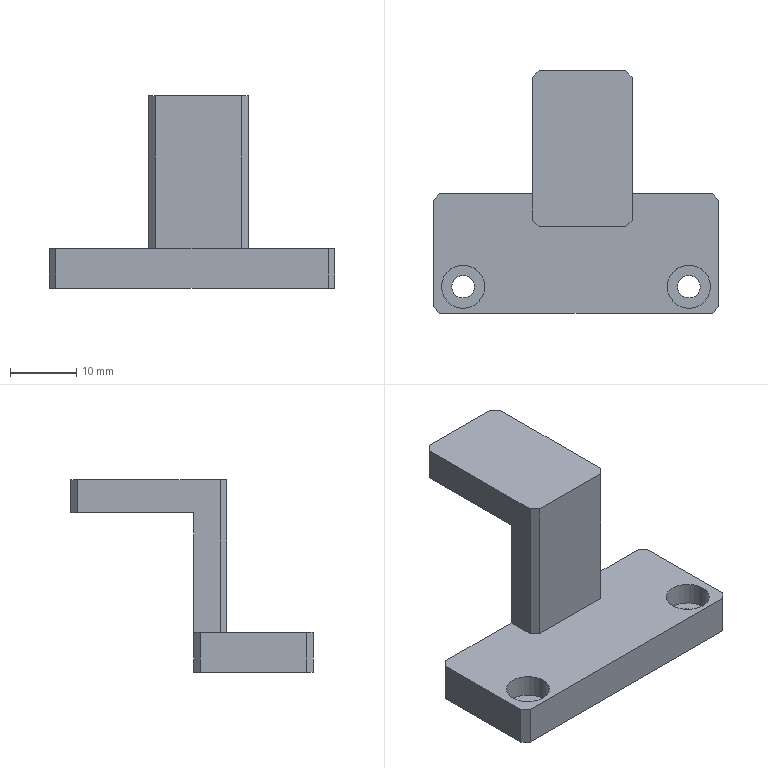Part | NX | 1 solid | 26 faces | box 43 x 36.5 x 29 mm | volume 7444 mm3 | plane 22 | cylinder 4 | commonest cylinder face diameters 3.4 x2 6.5 x2
STEP:
#1=CARTESIAN_POINT('',(21.5,8.,5.));
#2=VERTEX_POINT('',#1);
#3=CARTESIAN_POINT('',(20.5,9.,5.));
#4=VERTEX_POINT('',#3);
#5=CARTESIAN_POINT('',(14.75,14.75,5.));
#6=DIRECTION('',(-0.7071,0.7071,0.));
#7=VECTOR('',#6,1000.);
#8=LINE('',#5,#7);
#9=EDGE_CURVE('',#2,#4,#8,.T.);
#10=ORIENTED_EDGE('',*,*,#9,.F.);
#11=CARTESIAN_POINT('',(21.5,8.,-1.));
#12=VERTEX_POINT('',#11);
#13=CARTESIAN_POINT('',(21.5,8.,5.));
#14=DIRECTION('',(0.,0.,1.));
#15=VECTOR('',#14,1000.);
#16=LINE('',#13,#15);
#17=EDGE_CURVE('',#12,#2,#16,.T.);
#18=ORIENTED_EDGE('',*,*,#17,.F.);
#19=CARTESIAN_POINT('',(20.5,9.,-1.));
#20=VERTEX_POINT('',#19);
#21=CARTESIAN_POINT('',(20.5,9.,-1.));
#22=DIRECTION('',(0.7071,-0.7071,0.));
#23=VECTOR('',#22,1000.);
#24=LINE('',#21,#23);
#25=EDGE_CURVE('',#20,#12,#24,.T.);
#26=ORIENTED_EDGE('',*,*,#25,.F.);
#27=CARTESIAN_POINT('',(20.5,9.,5.));
#28=DIRECTION('',(0.,0.,-1.));
#29=VECTOR('',#28,1000.);
#30=LINE('',#27,#29);
#31=EDGE_CURVE('',#4,#20,#30,.T.);
#32=ORIENTED_EDGE('',*,*,#31,.F.);
#33=EDGE_LOOP('',(#10,#18,#26,#32));
#34=FACE_BOUND('',#33,.T.);
#35=CARTESIAN_POINT('',(20.5,9.,5.));
#36=DIRECTION('',(-0.7071,-0.7071,0.));
#37=DIRECTION('',(0.,0.,-1.));
#38=AXIS2_PLACEMENT_3D('',#35,#36,#37);
#39=PLANE('',#38);
#40=ADVANCED_FACE('',(#34),#39,.F.);
#41=CARTESIAN_POINT('',(20.5,-9.,5.));
#42=VERTEX_POINT('',#41);
#43=CARTESIAN_POINT('',(21.5,-8.,5.));
#44=VERTEX_POINT('',#43);
#45=CARTESIAN_POINT('',(14.75,-14.75,5.));
#46=DIRECTION('',(0.7071,0.7071,0.));
#47=VECTOR('',#46,1000.);
#48=LINE('',#45,#47);
#49=EDGE_CURVE('',#42,#44,#48,.T.);
#50=ORIENTED_EDGE('',*,*,#49,.F.);
#51=CARTESIAN_POINT('',(20.5,-9.,-1.));
#52=VERTEX_POINT('',#51);
#53=CARTESIAN_POINT('',(20.5,-9.,5.));
#54=DIRECTION('',(0.,0.,1.));
#55=VECTOR('',#54,1000.);
#56=LINE('',#53,#55);
#57=EDGE_CURVE('',#52,#42,#56,.T.);
#58=ORIENTED_EDGE('',*,*,#57,.F.);
#59=CARTESIAN_POINT('',(21.5,-8.,-1.));
#60=VERTEX_POINT('',#59);
#61=CARTESIAN_POINT('',(21.5,-8.,-1.));
#62=DIRECTION('',(-0.7071,-0.7071,0.));
#63=VECTOR('',#62,1000.);
#64=LINE('',#61,#63);
#65=EDGE_CURVE('',#60,#52,#64,.T.);
#66=ORIENTED_EDGE('',*,*,#65,.F.);
#67=CARTESIAN_POINT('',(21.5,-8.,5.));
#68=DIRECTION('',(0.,0.,-1.));
#69=VECTOR('',#68,1000.);
#70=LINE('',#67,#69);
#71=EDGE_CURVE('',#44,#60,#70,.T.);
#72=ORIENTED_EDGE('',*,*,#71,.F.);
#73=EDGE_LOOP('',(#50,#58,#66,#72));
#74=FACE_BOUND('',#73,.T.);
#75=CARTESIAN_POINT('',(21.5,-8.,5.));
#76=DIRECTION('',(-0.7071,0.7071,0.));
#77=DIRECTION('',(0.,0.,-1.));
#78=AXIS2_PLACEMENT_3D('',#75,#76,#77);
#79=PLANE('',#78);
#80=ADVANCED_FACE('',(#74),#79,.F.);
#81=CARTESIAN_POINT('',(-20.5,9.,5.));
#82=VERTEX_POINT('',#81);
#83=CARTESIAN_POINT('',(-21.5,8.,5.));
#84=VERTEX_POINT('',#83);
#85=CARTESIAN_POINT('',(-14.75,14.75,5.));
#86=DIRECTION('',(-0.7071,-0.7071,0.));
#87=VECTOR('',#86,1000.);
#88=LINE('',#85,#87);
#89=EDGE_CURVE('',#82,#84,#88,.T.);
#90=ORIENTED_EDGE('',*,*,#89,.F.);
#91=CARTESIAN_POINT('',(-20.5,9.,-1.));
#92=VERTEX_POINT('',#91);
#93=CARTESIAN_POINT('',(-20.5,9.,5.));
#94=DIRECTION('',(0.,0.,1.));
#95=VECTOR('',#94,1000.);
#96=LINE('',#93,#95);
#97=EDGE_CURVE('',#92,#82,#96,.T.);
#98=ORIENTED_EDGE('',*,*,#97,.F.);
#99=CARTESIAN_POINT('',(-21.5,8.,-1.));
#100=VERTEX_POINT('',#99);
#101=CARTESIAN_POINT('',(-21.5,8.,-1.));
#102=DIRECTION('',(0.7071,0.7071,0.));
#103=VECTOR('',#102,1000.);
#104=LINE('',#101,#103);
#105=EDGE_CURVE('',#100,#92,#104,.T.);
#106=ORIENTED_EDGE('',*,*,#105,.F.);
#107=CARTESIAN_POINT('',(-21.5,8.,5.));
#108=DIRECTION('',(0.,0.,-1.));
#109=VECTOR('',#108,1000.);
#110=LINE('',#107,#109);
#111=EDGE_CURVE('',#84,#100,#110,.T.);
#112=ORIENTED_EDGE('',*,*,#111,.F.);
#113=EDGE_LOOP('',(#90,#98,#106,#112));
#114=FACE_BOUND('',#113,.T.);
#115=CARTESIAN_POINT('',(-21.5,8.,5.));
#116=DIRECTION('',(0.7071,-0.7071,0.));
#117=DIRECTION('',(0.,0.,-1.));
#118=AXIS2_PLACEMENT_3D('',#115,#116,#117);
#119=PLANE('',#118);
#120=ADVANCED_FACE('',(#114),#119,.F.);
#121=CARTESIAN_POINT('',(-21.5,-8.,5.));
#122=VERTEX_POINT('',#121);
#123=CARTESIAN_POINT('',(-20.5,-9.,5.));
#124=VERTEX_POINT('',#123);
#125=CARTESIAN_POINT('',(-14.75,-14.75,5.));
#126=DIRECTION('',(0.7071,-0.7071,0.));
#127=VECTOR('',#126,1000.);
#128=LINE('',#125,#127);
#129=EDGE_CURVE('',#122,#124,#128,.T.);
#130=ORIENTED_EDGE('',*,*,#129,.F.);
#131=CARTESIAN_POINT('',(-21.5,-8.,-1.));
#132=VERTEX_POINT('',#131);
#133=CARTESIAN_POINT('',(-21.5,-8.,5.));
#134=DIRECTION('',(0.,0.,1.));
#135=VECTOR('',#134,1000.);
#136=LINE('',#133,#135);
#137=EDGE_CURVE('',#132,#122,#136,.T.);
#138=ORIENTED_EDGE('',*,*,#137,.F.);
#139=CARTESIAN_POINT('',(-20.5,-9.,-1.));
#140=VERTEX_POINT('',#139);
#141=CARTESIAN_POINT('',(-20.5,-9.,-1.));
#142=DIRECTION('',(-0.7071,0.7071,0.));
#143=VECTOR('',#142,1000.);
#144=LINE('',#141,#143);
#145=EDGE_CURVE('',#140,#132,#144,.T.);
#146=ORIENTED_EDGE('',*,*,#145,.F.);
#147=CARTESIAN_POINT('',(-20.5,-9.,5.));
#148=DIRECTION('',(0.,0.,-1.));
#149=VECTOR('',#148,1000.);
#150=LINE('',#147,#149);
#151=EDGE_CURVE('',#124,#140,#150,.T.);
#152=ORIENTED_EDGE('',*,*,#151,.F.);
#153=EDGE_LOOP('',(#130,#138,#146,#152));
#154=FACE_BOUND('',#153,.T.);
#155=CARTESIAN_POINT('',(-20.5,-9.,5.));
#156=DIRECTION('',(0.7071,0.7071,0.));
#157=DIRECTION('',(0.,0.,-1.));
#158=AXIS2_PLACEMENT_3D('',#155,#156,#157);
#159=PLANE('',#158);
#160=ADVANCED_FACE('',(#154),#159,.F.);
#161=CARTESIAN_POINT('',(-6.55,26.5,23.));
#162=VERTEX_POINT('',#161);
#163=CARTESIAN_POINT('',(-5.55,27.5,23.));
#164=VERTEX_POINT('',#163);
#165=CARTESIAN_POINT('',(-5.55,27.5,23.));
#166=DIRECTION('',(0.7071,0.7071,0.));
#167=VECTOR('',#166,1000.);
#168=LINE('',#165,#167);
#169=EDGE_CURVE('',#162,#164,#168,.T.);
#170=ORIENTED_EDGE('',*,*,#169,.F.);
#171=CARTESIAN_POINT('',(-6.55,26.5,28.));
#172=VERTEX_POINT('',#171);
#173=CARTESIAN_POINT('',(-6.55,26.5,28.));
#174=DIRECTION('',(0.,0.,-1.));
#175=VECTOR('',#174,1000.);
#176=LINE('',#173,#175);
#177=EDGE_CURVE('',#172,#162,#176,.T.);
#178=ORIENTED_EDGE('',*,*,#177,.F.);
#179=CARTESIAN_POINT('',(-5.55,27.5,28.));
#180=VERTEX_POINT('',#179);
#181=CARTESIAN_POINT('',(-16.525,16.525,28.));
#182=DIRECTION('',(-0.7071,-0.7071,0.));
#183=VECTOR('',#182,1000.);
#184=LINE('',#181,#183);
#185=EDGE_CURVE('',#180,#172,#184,.T.);
#186=ORIENTED_EDGE('',*,*,#185,.F.);
#187=CARTESIAN_POINT('',(-5.55,27.5,0.));
#188=DIRECTION('',(0.,0.,1.));
#189=VECTOR('',#188,1000.);
#190=LINE('',#187,#189);
#191=EDGE_CURVE('',#164,#180,#190,.T.);
#192=ORIENTED_EDGE('',*,*,#191,.F.);
#193=EDGE_LOOP('',(#170,#178,#186,#192));
#194=FACE_BOUND('',#193,.T.);
#195=CARTESIAN_POINT('',(-5.55,27.5,0.));
#196=DIRECTION('',(0.7071,-0.7071,0.));
#197=DIRECTION('',(0.,0.,1.));
#198=AXIS2_PLACEMENT_3D('',#195,#196,#197);
#199=PLANE('',#198);
#200=ADVANCED_FACE('',(#194),#199,.F.);
#201=CARTESIAN_POINT('',(8.45,26.5,28.));
#202=VERTEX_POINT('',#201);
#203=CARTESIAN_POINT('',(7.45,27.5,28.));
#204=VERTEX_POINT('',#203);
#205=CARTESIAN_POINT('',(17.475,17.475,28.));
#206=DIRECTION('',(-0.7071,0.7071,0.));
#207=VECTOR('',#206,1000.);
#208=LINE('',#205,#207);
#209=EDGE_CURVE('',#202,#204,#208,.T.);
#210=ORIENTED_EDGE('',*,*,#209,.F.);
#211=CARTESIAN_POINT('',(8.45,26.5,23.));
#212=VERTEX_POINT('',#211);
#213=CARTESIAN_POINT('',(8.45,26.5,28.));
#214=DIRECTION('',(0.,0.,1.));
#215=VECTOR('',#214,1000.);
#216=LINE('',#213,#215);
#217=EDGE_CURVE('',#212,#202,#216,.T.);
#218=ORIENTED_EDGE('',*,*,#217,.F.);
#219=CARTESIAN_POINT('',(7.45,27.5,23.));
#220=VERTEX_POINT('',#219);
#221=CARTESIAN_POINT('',(7.45,27.5,23.));
#222=DIRECTION('',(0.7071,-0.7071,0.));
#223=VECTOR('',#222,1000.);
#224=LINE('',#221,#223);
#225=EDGE_CURVE('',#220,#212,#224,.T.);
#226=ORIENTED_EDGE('',*,*,#225,.F.);
#227=CARTESIAN_POINT('',(7.45,27.5,0.));
#228=DIRECTION('',(0.,0.,-1.));
#229=VECTOR('',#228,1000.);
#230=LINE('',#227,#229);
#231=EDGE_CURVE('',#204,#220,#230,.T.);
#232=ORIENTED_EDGE('',*,*,#231,.F.);
#233=EDGE_LOOP('',(#210,#218,#226,#232));
#234=FACE_BOUND('',#233,.T.);
#235=CARTESIAN_POINT('',(7.45,27.5,0.));
#236=DIRECTION('',(-0.7071,-0.7071,0.));
#237=DIRECTION('',(0.,0.,-1.));
#238=AXIS2_PLACEMENT_3D('',#235,#236,#237);
#239=PLANE('',#238);
#240=ADVANCED_FACE('',(#234),#239,.F.);
#241=CARTESIAN_POINT('',(-6.55,5.,28.));
#242=VERTEX_POINT('',#241);
#243=CARTESIAN_POINT('',(-5.55,4.,28.));
#244=VERTEX_POINT('',#243);
#245=CARTESIAN_POINT('',(-0.775,-0.775,28.));
#246=DIRECTION('',(0.7071,-0.7071,0.));
#247=VECTOR('',#246,1000.);
#248=LINE('',#245,#247);
#249=EDGE_CURVE('',#242,#244,#248,.T.);
#250=ORIENTED_EDGE('',*,*,#249,.F.);
#251=CARTESIAN_POINT('',(-6.55,5.,5.));
#252=VERTEX_POINT('',#251);
#253=CARTESIAN_POINT('',(-6.55,5.,28.));
#254=DIRECTION('',(0.,0.,1.));
#255=VECTOR('',#254,1000.);
#256=LINE('',#253,#255);
#257=EDGE_CURVE('',#252,#242,#256,.T.);
#258=ORIENTED_EDGE('',*,*,#257,.F.);
#259=CARTESIAN_POINT('',(-5.55,4.,5.));
#260=VERTEX_POINT('',#259);
#261=CARTESIAN_POINT('',(-5.55,4.,5.));
#262=DIRECTION('',(-0.7071,0.7071,0.));
#263=VECTOR('',#262,1000.);
#264=LINE('',#261,#263);
#265=EDGE_CURVE('',#260,#252,#264,.T.);
#266=ORIENTED_EDGE('',*,*,#265,.F.);
#267=CARTESIAN_POINT('',(-5.55,4.,28.));
#268=DIRECTION('',(0.,0.,-1.));
#269=VECTOR('',#268,1000.);
#270=LINE('',#267,#269);
#271=EDGE_CURVE('',#244,#260,#270,.T.);
#272=ORIENTED_EDGE('',*,*,#271,.F.);
#273=EDGE_LOOP('',(#250,#258,#266,#272));
#274=FACE_BOUND('',#273,.T.);
#275=CARTESIAN_POINT('',(-5.55,4.,28.));
#276=DIRECTION('',(0.7071,0.7071,0.));
#277=DIRECTION('',(0.,0.,-1.));
#278=AXIS2_PLACEMENT_3D('',#275,#276,#277);
#279=PLANE('',#278);
#280=ADVANCED_FACE('',(#274),#279,.F.);
#281=CARTESIAN_POINT('',(7.45,4.,28.));
#282=VERTEX_POINT('',#281);
#283=CARTESIAN_POINT('',(8.45,5.,28.));
#284=VERTEX_POINT('',#283);
#285=CARTESIAN_POINT('',(1.725,-1.725,28.));
#286=DIRECTION('',(0.7071,0.7071,0.));
#287=VECTOR('',#286,1000.);
#288=LINE('',#285,#287);
#289=EDGE_CURVE('',#282,#284,#288,.T.);
#290=ORIENTED_EDGE('',*,*,#289,.F.);
#291=CARTESIAN_POINT('',(7.45,4.,5.));
#292=VERTEX_POINT('',#291);
#293=CARTESIAN_POINT('',(7.45,4.,28.));
#294=DIRECTION('',(0.,0.,1.));
#295=VECTOR('',#294,1000.);
#296=LINE('',#293,#295);
#297=EDGE_CURVE('',#292,#282,#296,.T.);
#298=ORIENTED_EDGE('',*,*,#297,.F.);
#299=CARTESIAN_POINT('',(8.45,5.,5.));
#300=VERTEX_POINT('',#299);
#301=CARTESIAN_POINT('',(8.45,5.,5.));
#302=DIRECTION('',(-0.7071,-0.7071,0.));
#303=VECTOR('',#302,1000.);
#304=LINE('',#301,#303);
#305=EDGE_CURVE('',#300,#292,#304,.T.);
#306=ORIENTED_EDGE('',*,*,#305,.F.);
#307=CARTESIAN_POINT('',(8.45,5.,28.));
#308=DIRECTION('',(0.,0.,-1.));
#309=VECTOR('',#308,1000.);
#310=LINE('',#307,#309);
#311=EDGE_CURVE('',#284,#300,#310,.T.);
#312=ORIENTED_EDGE('',*,*,#311,.F.);
#313=EDGE_LOOP('',(#290,#298,#306,#312));
#314=FACE_BOUND('',#313,.T.);
#315=CARTESIAN_POINT('',(8.45,5.,28.));
#316=DIRECTION('',(-0.7071,0.7071,0.));
#317=DIRECTION('',(0.,0.,-1.));
#318=AXIS2_PLACEMENT_3D('',#315,#316,#317);
#319=PLANE('',#318);
#320=ADVANCED_FACE('',(#314),#319,.F.);
#321=CARTESIAN_POINT('',(-6.55,27.5,28.));
#322=DIRECTION('',(1.,0.,0.));
#323=VECTOR('',#322,1000.);
#324=LINE('',#321,#323);
#325=EDGE_CURVE('',#180,#204,#324,.T.);
#326=ORIENTED_EDGE('',*,*,#325,.T.);
#327=ORIENTED_EDGE('',*,*,#231,.T.);
#328=CARTESIAN_POINT('',(-6.55,27.5,23.));
#329=DIRECTION('',(-1.,0.,0.));
#330=VECTOR('',#329,1000.);
#331=LINE('',#328,#330);
#332=EDGE_CURVE('',#220,#164,#331,.T.);
#333=ORIENTED_EDGE('',*,*,#332,.T.);
#334=ORIENTED_EDGE('',*,*,#191,.T.);
#335=EDGE_LOOP('',(#326,#327,#333,#334));
#336=FACE_BOUND('',#335,.T.);
#337=CARTESIAN_POINT('',(0.,27.5,0.));
#338=DIRECTION('',(0.,-1.,0.));
#339=DIRECTION('',(1.,0.,0.));
#340=AXIS2_PLACEMENT_3D('',#337,#338,#339);
#341=PLANE('',#340);
#342=ADVANCED_FACE('',(#336),#341,.F.);
#343=ORIENTED_EDGE('',*,*,#332,.F.);
#344=ORIENTED_EDGE('',*,*,#225,.T.);
#345=CARTESIAN_POINT('',(8.45,9.,23.));
#346=VERTEX_POINT('',#345);
#347=CARTESIAN_POINT('',(8.45,27.5,23.));
#348=DIRECTION('',(0.,-1.,0.));
#349=VECTOR('',#348,1000.);
#350=LINE('',#347,#349);
#351=EDGE_CURVE('',#212,#346,#350,.T.);
#352=ORIENTED_EDGE('',*,*,#351,.T.);
#353=CARTESIAN_POINT('',(-6.55,9.,23.));
#354=VERTEX_POINT('',#353);
#355=CARTESIAN_POINT('',(-6.55,9.,23.));
#356=DIRECTION('',(-1.,0.,0.));
#357=VECTOR('',#356,1000.);
#358=LINE('',#355,#357);
#359=EDGE_CURVE('',#346,#354,#358,.T.);
#360=ORIENTED_EDGE('',*,*,#359,.T.);
#361=CARTESIAN_POINT('',(-6.55,27.5,23.));
#362=DIRECTION('',(0.,-1.,0.));
#363=VECTOR('',#362,1000.);
#364=LINE('',#361,#363);
#365=EDGE_CURVE('',#162,#354,#364,.T.);
#366=ORIENTED_EDGE('',*,*,#365,.F.);
#367=ORIENTED_EDGE('',*,*,#169,.T.);
#368=EDGE_LOOP('',(#343,#344,#352,#360,#366,#367));
#369=FACE_BOUND('',#368,.T.);
#370=CARTESIAN_POINT('',(-6.55,27.5,23.));
#371=DIRECTION('',(0.,0.,1.));
#372=DIRECTION('',(1.,0.,0.));
#373=AXIS2_PLACEMENT_3D('',#370,#371,#372);
#374=PLANE('',#373);
#375=ADVANCED_FACE('',(#369),#374,.F.);
#376=CARTESIAN_POINT('',(-6.55,4.,28.));
#377=DIRECTION('',(1.,0.,0.));
#378=VECTOR('',#377,1000.);
#379=LINE('',#376,#378);
#380=EDGE_CURVE('',#244,#282,#379,.T.);
#381=ORIENTED_EDGE('',*,*,#380,.T.);
#382=ORIENTED_EDGE('',*,*,#289,.T.);
#383=CARTESIAN_POINT('',(8.45,9.,28.));
#384=DIRECTION('',(0.,1.,0.));
#385=VECTOR('',#384,1000.);
#386=LINE('',#383,#385);
#387=EDGE_CURVE('',#284,#202,#386,.T.);
#388=ORIENTED_EDGE('',*,*,#387,.T.);
#389=ORIENTED_EDGE('',*,*,#209,.T.);
#390=ORIENTED_EDGE('',*,*,#325,.F.);
#391=ORIENTED_EDGE('',*,*,#185,.T.);
#392=CARTESIAN_POINT('',(-6.55,9.,28.));
#393=DIRECTION('',(0.,-1.,0.));
#394=VECTOR('',#393,1000.);
#395=LINE('',#392,#394);
#396=EDGE_CURVE('',#172,#242,#395,.T.);
#397=ORIENTED_EDGE('',*,*,#396,.T.);
#398=ORIENTED_EDGE('',*,*,#249,.T.);
#399=EDGE_LOOP('',(#381,#382,#388,#389,#390,#391,#397,#398));
#400=FACE_BOUND('',#399,.T.);
#401=CARTESIAN_POINT('',(0.,0.,28.));
#402=DIRECTION('',(0.,0.,1.));
#403=DIRECTION('',(1.,0.,0.));
#404=AXIS2_PLACEMENT_3D('',#401,#402,#403);
#405=PLANE('',#404);
#406=ADVANCED_FACE('',(#400),#405,.T.);
#407=ORIENTED_EDGE('',*,*,#387,.F.);
#408=ORIENTED_EDGE('',*,*,#311,.T.);
#409=CARTESIAN_POINT('',(8.45,9.,5.));
#410=VERTEX_POINT('',#409);
#411=CARTESIAN_POINT('',(8.45,9.,5.));
#412=DIRECTION('',(0.,1.,0.));
#413=VECTOR('',#412,1000.);
#414=LINE('',#411,#413);
#415=EDGE_CURVE('',#300,#410,#414,.T.);
#416=ORIENTED_EDGE('',*,*,#415,.T.);
#417=CARTESIAN_POINT('',(8.45,9.,28.));
#418=DIRECTION('',(0.,0.,-1.));
#419=VECTOR('',#418,1000.);
#420=LINE('',#417,#419);
#421=EDGE_CURVE('',#346,#410,#420,.T.);
#422=ORIENTED_EDGE('',*,*,#421,.F.);
#423=ORIENTED_EDGE('',*,*,#351,.F.);
#424=ORIENTED_EDGE('',*,*,#217,.T.);
#425=EDGE_LOOP('',(#407,#408,#416,#422,#423,#424));
#426=FACE_BOUND('',#425,.T.);
#427=CARTESIAN_POINT('',(8.45,9.,28.));
#428=DIRECTION('',(-1.,0.,0.));
#429=DIRECTION('',(0.,0.,1.));
#430=AXIS2_PLACEMENT_3D('',#427,#428,#429);
#431=PLANE('',#430);
#432=ADVANCED_FACE('',(#426),#431,.F.);
#433=CARTESIAN_POINT('',(-6.55,4.,5.));
#434=DIRECTION('',(1.,0.,0.));
#435=VECTOR('',#434,1000.);
#436=LINE('',#433,#435);
#437=EDGE_CURVE('',#260,#292,#436,.T.);
#438=ORIENTED_EDGE('',*,*,#437,.T.);
#439=ORIENTED_EDGE('',*,*,#297,.T.);
#440=ORIENTED_EDGE('',*,*,#380,.F.);
#441=ORIENTED_EDGE('',*,*,#271,.T.);
#442=EDGE_LOOP('',(#438,#439,#440,#441));
#443=FACE_BOUND('',#442,.T.);
#444=CARTESIAN_POINT('',(-6.55,4.,28.));
#445=DIRECTION('',(0.,1.,0.));
#446=DIRECTION('',(-1.,0.,0.));
#447=AXIS2_PLACEMENT_3D('',#444,#445,#446);
#448=PLANE('',#447);
#449=ADVANCED_FACE('',(#443),#448,.F.);
#450=CARTESIAN_POINT('',(-6.55,9.,5.));
#451=VERTEX_POINT('',#450);
#452=CARTESIAN_POINT('',(-6.55,9.,5.));
#453=DIRECTION('',(0.,-1.,0.));
#454=VECTOR('',#453,1000.);
#455=LINE('',#452,#454);
#456=EDGE_CURVE('',#451,#252,#455,.T.);
#457=ORIENTED_EDGE('',*,*,#456,.T.);
#458=ORIENTED_EDGE('',*,*,#257,.T.);
#459=ORIENTED_EDGE('',*,*,#396,.F.);
#460=ORIENTED_EDGE('',*,*,#177,.T.);
#461=ORIENTED_EDGE('',*,*,#365,.T.);
#462=CARTESIAN_POINT('',(-6.55,9.,28.));
#463=DIRECTION('',(0.,0.,-1.));
#464=VECTOR('',#463,1000.);
#465=LINE('',#462,#464);
#466=EDGE_CURVE('',#354,#451,#465,.T.);
#467=ORIENTED_EDGE('',*,*,#466,.T.);
#468=EDGE_LOOP('',(#457,#458,#459,#460,#461,#467));
#469=FACE_BOUND('',#468,.T.);
#470=CARTESIAN_POINT('',(-6.55,9.,28.));
#471=DIRECTION('',(1.,0.,0.));
#472=DIRECTION('',(0.,0.,-1.));
#473=AXIS2_PLACEMENT_3D('',#470,#471,#472);
#474=PLANE('',#473);
#475=ADVANCED_FACE('',(#469),#474,.F.);
#476=CARTESIAN_POINT('',(-20.25,-5.,1.6));
#477=VERTEX_POINT('',#476);
#478=CARTESIAN_POINT('',(-17.,-5.,1.6));
#479=DIRECTION('',(0.,0.,1.));
#480=DIRECTION('',(-1.,0.,0.));
#481=AXIS2_PLACEMENT_3D('',#478,#479,#480);
#482=CIRCLE('',#481,3.25);
#483=EDGE_CURVE('',#477,#477,#482,.T.);
#484=ORIENTED_EDGE('',*,*,#483,.T.);
#485=EDGE_LOOP('',(#484));
#486=FACE_BOUND('',#485,.T.);
#487=CARTESIAN_POINT('',(-18.7,-5.,1.6));
#488=VERTEX_POINT('',#487);
#489=CARTESIAN_POINT('',(-17.,-5.,1.6));
#490=DIRECTION('',(0.,0.,1.));
#491=DIRECTION('',(-1.,0.,0.));
#492=AXIS2_PLACEMENT_3D('',#489,#490,#491);
#493=CIRCLE('',#492,1.7);
#494=EDGE_CURVE('',#488,#488,#493,.T.);
#495=ORIENTED_EDGE('',*,*,#494,.F.);
#496=EDGE_LOOP('',(#495));
#497=FACE_BOUND('',#496,.T.);
#498=CARTESIAN_POINT('',(18.7,-5.,1.6));
#499=DIRECTION('',(0.,0.,-1.));
#500=DIRECTION('',(-1.,0.,0.));
#501=AXIS2_PLACEMENT_3D('',#498,#499,#500);
#502=PLANE('',#501);
#503=ADVANCED_FACE('',(#486,#497),#502,.F.);
#504=CARTESIAN_POINT('',(20.25,-5.,1.6));
#505=VERTEX_POINT('',#504);
#506=CARTESIAN_POINT('',(17.,-5.,1.6));
#507=DIRECTION('',(0.,0.,1.));
#508=DIRECTION('',(1.,0.,0.));
#509=AXIS2_PLACEMENT_3D('',#506,#507,#508);
#510=CIRCLE('',#509,3.25);
#511=EDGE_CURVE('',#505,#505,#510,.T.);
#512=ORIENTED_EDGE('',*,*,#511,.T.);
#513=EDGE_LOOP('',(#512));
#514=FACE_BOUND('',#513,.T.);
#515=CARTESIAN_POINT('',(18.7,-5.,1.6));
#516=VERTEX_POINT('',#515);
#517=CARTESIAN_POINT('',(17.,-5.,1.6));
#518=DIRECTION('',(0.,0.,1.));
#519=DIRECTION('',(1.,0.,0.));
#520=AXIS2_PLACEMENT_3D('',#517,#518,#519);
#521=CIRCLE('',#520,1.7);
#522=EDGE_CURVE('',#516,#516,#521,.T.);
#523=ORIENTED_EDGE('',*,*,#522,.F.);
#524=EDGE_LOOP('',(#523));
#525=FACE_BOUND('',#524,.T.);
#526=CARTESIAN_POINT('',(18.7,-5.,1.6));
#527=DIRECTION('',(0.,0.,-1.));
#528=DIRECTION('',(-1.,0.,0.));
#529=AXIS2_PLACEMENT_3D('',#526,#527,#528);
#530=PLANE('',#529);
#531=ADVANCED_FACE('',(#514,#525),#530,.F.);
#532=CARTESIAN_POINT('',(-21.5,-9.,-1.));
#533=DIRECTION('',(1.,0.,0.));
#534=VECTOR('',#533,1000.);
#535=LINE('',#532,#534);
#536=EDGE_CURVE('',#140,#52,#535,.T.);
#537=ORIENTED_EDGE('',*,*,#536,.F.);
#538=ORIENTED_EDGE('',*,*,#145,.T.);
#539=CARTESIAN_POINT('',(-21.5,-9.,-1.));
#540=DIRECTION('',(0.,-1.,0.));
#541=VECTOR('',#540,1000.);
#542=LINE('',#539,#541);
#543=EDGE_CURVE('',#100,#132,#542,.T.);
#544=ORIENTED_EDGE('',*,*,#543,.F.);
#545=ORIENTED_EDGE('',*,*,#105,.T.);
#546=CARTESIAN_POINT('',(22.5,9.,-1.));
#547=DIRECTION('',(-1.,0.,0.));
#548=VECTOR('',#547,1000.);
#549=LINE('',#546,#548);
#550=EDGE_CURVE('',#20,#92,#549,.T.);
#551=ORIENTED_EDGE('',*,*,#550,.F.);
#552=ORIENTED_EDGE('',*,*,#25,.T.);
#553=CARTESIAN_POINT('',(21.5,-9.,-1.));
#554=DIRECTION('',(0.,-1.,0.));
#555=VECTOR('',#554,1000.);
#556=LINE('',#553,#555);
#557=EDGE_CURVE('',#12,#60,#556,.T.);
#558=ORIENTED_EDGE('',*,*,#557,.T.);
#559=ORIENTED_EDGE('',*,*,#65,.T.);
#560=EDGE_LOOP('',(#537,#538,#544,#545,#551,#552,#558,#559));
#561=FACE_BOUND('',#560,.T.);
#562=CARTESIAN_POINT('',(18.7,-5.,-1.));
#563=VERTEX_POINT('',#562);
#564=CARTESIAN_POINT('',(17.,-5.,-1.));
#565=DIRECTION('',(0.,0.,1.));
#566=DIRECTION('',(1.,0.,0.));
#567=AXIS2_PLACEMENT_3D('',#564,#565,#566);
#568=CIRCLE('',#567,1.7);
#569=EDGE_CURVE('',#563,#563,#568,.T.);
#570=ORIENTED_EDGE('',*,*,#569,.T.);
#571=EDGE_LOOP('',(#570));
#572=FACE_BOUND('',#571,.T.);
#573=CARTESIAN_POINT('',(-15.3,-5.,-1.));
#574=VERTEX_POINT('',#573);
#575=CARTESIAN_POINT('',(-17.,-5.,-1.));
#576=DIRECTION('',(0.,0.,1.));
#577=DIRECTION('',(1.,0.,0.));
#578=AXIS2_PLACEMENT_3D('',#575,#576,#577);
#579=CIRCLE('',#578,1.7);
#580=EDGE_CURVE('',#574,#574,#579,.T.);
#581=ORIENTED_EDGE('',*,*,#580,.T.);
#582=EDGE_LOOP('',(#581));
#583=FACE_BOUND('',#582,.T.);
#584=CARTESIAN_POINT('',(-21.5,-9.,-1.));
#585=DIRECTION('',(0.,0.,1.));
#586=DIRECTION('',(1.,0.,0.));
#587=AXIS2_PLACEMENT_3D('',#584,#585,#586);
#588=PLANE('',#587);
#589=ADVANCED_FACE('',(#561,#572,#583),#588,.F.);
#590=CARTESIAN_POINT('',(20.25,-5.,5.));
#591=VERTEX_POINT('',#590);
#592=CARTESIAN_POINT('',(17.,-5.,5.));
#593=DIRECTION('',(0.,0.,1.));
#594=DIRECTION('',(1.,0.,0.));
#595=AXIS2_PLACEMENT_3D('',#592,#593,#594);
#596=CIRCLE('',#595,3.25);
#597=EDGE_CURVE('',#591,#591,#596,.T.);
#598=ORIENTED_EDGE('',*,*,#597,.F.);
#599=EDGE_LOOP('',(#598));
#600=FACE_BOUND('',#599,.T.);
#601=CARTESIAN_POINT('',(-13.75,-5.,5.));
#602=VERTEX_POINT('',#601);
#603=CARTESIAN_POINT('',(-17.,-5.,5.));
#604=DIRECTION('',(0.,0.,1.));
#605=DIRECTION('',(1.,0.,0.));
#606=AXIS2_PLACEMENT_3D('',#603,#604,#605);
#607=CIRCLE('',#606,3.25);
#608=EDGE_CURVE('',#602,#602,#607,.T.);
#609=ORIENTED_EDGE('',*,*,#608,.F.);
#610=EDGE_LOOP('',(#609));
#611=FACE_BOUND('',#610,.T.);
#612=CARTESIAN_POINT('',(-21.5,-9.,5.));
#613=DIRECTION('',(0.,-1.,0.));
#614=VECTOR('',#613,1000.);
#615=LINE('',#612,#614);
#616=EDGE_CURVE('',#84,#122,#615,.T.);
#617=ORIENTED_EDGE('',*,*,#616,.T.);
#618=ORIENTED_EDGE('',*,*,#129,.T.);
#619=CARTESIAN_POINT('',(21.5,-9.,5.));
#620=DIRECTION('',(1.,0.,0.));
#621=VECTOR('',#620,1000.);
#622=LINE('',#619,#621);
#623=EDGE_CURVE('',#124,#42,#622,.T.);
#624=ORIENTED_EDGE('',*,*,#623,.T.);
#625=ORIENTED_EDGE('',*,*,#49,.T.);
#626=CARTESIAN_POINT('',(21.5,-9.,5.));
#627=DIRECTION('',(0.,1.,0.));
#628=VECTOR('',#627,1000.);
#629=LINE('',#626,#628);
#630=EDGE_CURVE('',#44,#2,#629,.T.);
#631=ORIENTED_EDGE('',*,*,#630,.T.);
#632=ORIENTED_EDGE('',*,*,#9,.T.);
#633=CARTESIAN_POINT('',(21.5,9.,5.));
#634=DIRECTION('',(-1.,0.,0.));
#635=VECTOR('',#634,1000.);
#636=LINE('',#633,#635);
#637=EDGE_CURVE('',#4,#410,#636,.T.);
#638=ORIENTED_EDGE('',*,*,#637,.T.);
#639=ORIENTED_EDGE('',*,*,#415,.F.);
#640=ORIENTED_EDGE('',*,*,#305,.T.);
#641=ORIENTED_EDGE('',*,*,#437,.F.);
#642=ORIENTED_EDGE('',*,*,#265,.T.);
#643=ORIENTED_EDGE('',*,*,#456,.F.);
#644=CARTESIAN_POINT('',(21.5,9.,5.));
#645=DIRECTION('',(-1.,0.,0.));
#646=VECTOR('',#645,1000.);
#647=LINE('',#644,#646);
#648=EDGE_CURVE('',#451,#82,#647,.T.);
#649=ORIENTED_EDGE('',*,*,#648,.T.);
#650=ORIENTED_EDGE('',*,*,#89,.T.);
#651=EDGE_LOOP('',(#617,#618,#624,#625,#631,#632,#638,#639,#640,#641,#642,#643,#649,#650));
#652=FACE_BOUND('',#651,.T.);
#653=CARTESIAN_POINT('',(0.,0.,5.));
#654=DIRECTION('',(0.,0.,1.));
#655=DIRECTION('',(1.,0.,0.));
#656=AXIS2_PLACEMENT_3D('',#653,#654,#655);
#657=PLANE('',#656);
#658=ADVANCED_FACE('',(#600,#611,#652),#657,.T.);
#659=ORIENTED_EDGE('',*,*,#630,.F.);
#660=ORIENTED_EDGE('',*,*,#71,.T.);
#661=ORIENTED_EDGE('',*,*,#557,.F.);
#662=ORIENTED_EDGE('',*,*,#17,.T.);
#663=EDGE_LOOP('',(#659,#660,#661,#662));
#664=FACE_BOUND('',#663,.T.);
#665=CARTESIAN_POINT('',(21.5,-9.,5.));
#666=DIRECTION('',(-1.,0.,0.));
#667=DIRECTION('',(0.,0.,1.));
#668=AXIS2_PLACEMENT_3D('',#665,#666,#667);
#669=PLANE('',#668);
#670=ADVANCED_FACE('',(#664),#669,.F.);
#671=ORIENTED_EDGE('',*,*,#623,.F.);
#672=ORIENTED_EDGE('',*,*,#151,.T.);
#673=ORIENTED_EDGE('',*,*,#536,.T.);
#674=ORIENTED_EDGE('',*,*,#57,.T.);
#675=EDGE_LOOP('',(#671,#672,#673,#674));
#676=FACE_BOUND('',#675,.T.);
#677=CARTESIAN_POINT('',(21.5,-9.,5.));
#678=DIRECTION('',(0.,1.,0.));
#679=DIRECTION('',(-1.,0.,0.));
#680=AXIS2_PLACEMENT_3D('',#677,#678,#679);
#681=PLANE('',#680);
#682=ADVANCED_FACE('',(#676),#681,.F.);
#683=ORIENTED_EDGE('',*,*,#543,.T.);
#684=ORIENTED_EDGE('',*,*,#137,.T.);
#685=ORIENTED_EDGE('',*,*,#616,.F.);
#686=ORIENTED_EDGE('',*,*,#111,.T.);
#687=EDGE_LOOP('',(#683,#684,#685,#686));
#688=FACE_BOUND('',#687,.T.);
#689=CARTESIAN_POINT('',(-21.5,-9.,5.));
#690=DIRECTION('',(1.,0.,0.));
#691=DIRECTION('',(0.,0.,-1.));
#692=AXIS2_PLACEMENT_3D('',#689,#690,#691);
#693=PLANE('',#692);
#694=ADVANCED_FACE('',(#688),#693,.F.);
#695=ORIENTED_EDGE('',*,*,#550,.T.);
#696=ORIENTED_EDGE('',*,*,#97,.T.);
#697=ORIENTED_EDGE('',*,*,#648,.F.);
#698=ORIENTED_EDGE('',*,*,#466,.F.);
#699=ORIENTED_EDGE('',*,*,#359,.F.);
#700=ORIENTED_EDGE('',*,*,#421,.T.);
#701=ORIENTED_EDGE('',*,*,#637,.F.);
#702=ORIENTED_EDGE('',*,*,#31,.T.);
#703=EDGE_LOOP('',(#695,#696,#697,#698,#699,#700,#701,#702));
#704=FACE_BOUND('',#703,.T.);
#705=CARTESIAN_POINT('',(21.5,9.,5.));
#706=DIRECTION('',(0.,-1.,0.));
#707=DIRECTION('',(1.,0.,0.));
#708=AXIS2_PLACEMENT_3D('',#705,#706,#707);
#709=PLANE('',#708);
#710=ADVANCED_FACE('',(#704),#709,.F.);
#711=ORIENTED_EDGE('',*,*,#569,.F.);
#712=EDGE_LOOP('',(#711));
#713=FACE_BOUND('',#712,.T.);
#714=ORIENTED_EDGE('',*,*,#522,.T.);
#715=EDGE_LOOP('',(#714));
#716=FACE_BOUND('',#715,.T.);
#717=CARTESIAN_POINT('',(17.,-5.,5.));
#718=DIRECTION('',(0.,0.,1.));
#719=DIRECTION('',(1.,0.,0.));
#720=AXIS2_PLACEMENT_3D('',#717,#718,#719);
#721=CYLINDRICAL_SURFACE('',#720,1.7);
#722=ADVANCED_FACE('',(#713,#716),#721,.F.);
#723=ORIENTED_EDGE('',*,*,#511,.F.);
#724=EDGE_LOOP('',(#723));
#725=FACE_BOUND('',#724,.T.);
#726=ORIENTED_EDGE('',*,*,#597,.T.);
#727=EDGE_LOOP('',(#726));
#728=FACE_BOUND('',#727,.T.);
#729=CARTESIAN_POINT('',(17.,-5.,5.));
#730=DIRECTION('',(0.,0.,1.));
#731=DIRECTION('',(1.,0.,0.));
#732=AXIS2_PLACEMENT_3D('',#729,#730,#731);
#733=CYLINDRICAL_SURFACE('',#732,3.25);
#734=ADVANCED_FACE('',(#725,#728),#733,.F.);
#735=ORIENTED_EDGE('',*,*,#580,.F.);
#736=EDGE_LOOP('',(#735));
#737=FACE_BOUND('',#736,.T.);
#738=ORIENTED_EDGE('',*,*,#494,.T.);
#739=EDGE_LOOP('',(#738));
#740=FACE_BOUND('',#739,.T.);
#741=CARTESIAN_POINT('',(-17.,-5.,5.));
#742=DIRECTION('',(0.,0.,1.));
#743=DIRECTION('',(1.,0.,0.));
#744=AXIS2_PLACEMENT_3D('',#741,#742,#743);
#745=CYLINDRICAL_SURFACE('',#744,1.7);
#746=ADVANCED_FACE('',(#737,#740),#745,.F.);
#747=ORIENTED_EDGE('',*,*,#483,.F.);
#748=EDGE_LOOP('',(#747));
#749=FACE_BOUND('',#748,.T.);
#750=ORIENTED_EDGE('',*,*,#608,.T.);
#751=EDGE_LOOP('',(#750));
#752=FACE_BOUND('',#751,.T.);
#753=CARTESIAN_POINT('',(-17.,-5.,5.));
#754=DIRECTION('',(0.,0.,1.));
#755=DIRECTION('',(1.,0.,0.));
#756=AXIS2_PLACEMENT_3D('',#753,#754,#755);
#757=CYLINDRICAL_SURFACE('',#756,3.25);
#758=ADVANCED_FACE('',(#749,#752),#757,.F.);
#759=CLOSED_SHELL('',(#40,#80,#120,#160,#200,#240,#280,#320,#342,#375,#406,#432,#449,#475,#503,#531,#589,#658,#670,#682,#694,#710,#722,#734,#746,#758));
#760=MANIFOLD_SOLID_BREP('',#759);
#761=(LENGTH_UNIT()NAMED_UNIT(*)SI_UNIT(.MILLI.,.METRE.));
#762=UNCERTAINTY_MEASURE_WITH_UNIT(LENGTH_MEASURE(0.00001),#761,'','');
#763=(NAMED_UNIT(*)PLANE_ANGLE_UNIT()SI_UNIT($,.RADIAN.));
#764=(NAMED_UNIT(*)SI_UNIT($,.STERADIAN.)SOLID_ANGLE_UNIT());
#765=(GEOMETRIC_REPRESENTATION_CONTEXT(3)GLOBAL_UNCERTAINTY_ASSIGNED_CONTEXT((#762))GLOBAL_UNIT_ASSIGNED_CONTEXT((#761,#763,#764))REPRESENTATION_CONTEXT('',''));
#766=ADVANCED_BREP_SHAPE_REPRESENTATION('',(#760),#765);